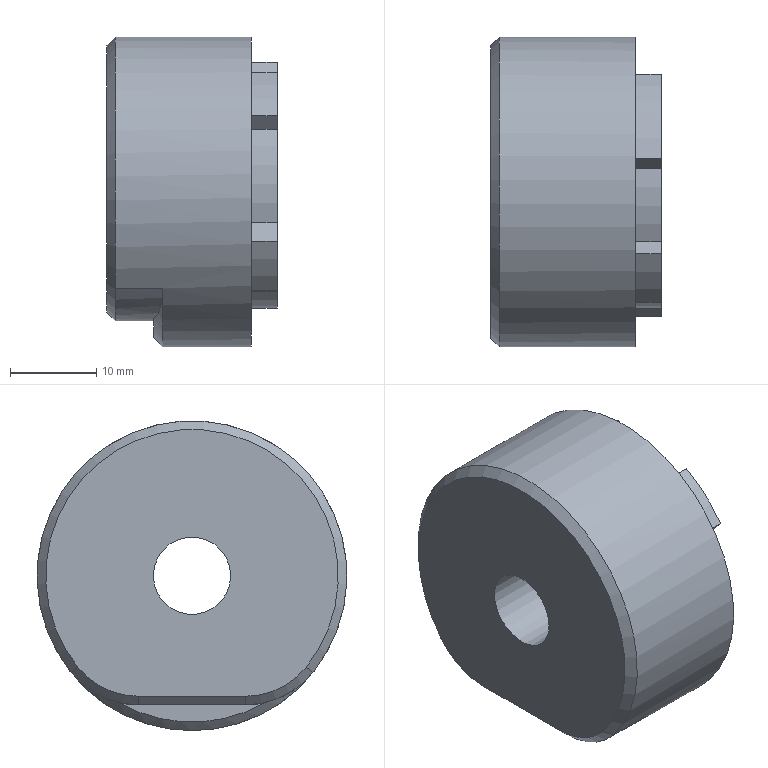Part | STEP file | solid 271 | 1 solid | 32 faces | box 19.849 x 36 x 36 mm | volume 16717 mm3 | plane 15 | cylinder 13 | cone 4 | commonest cylinder face diameters 27.135 x4 31.155 x4 20 x2 9 x1 14 x1 36 x1